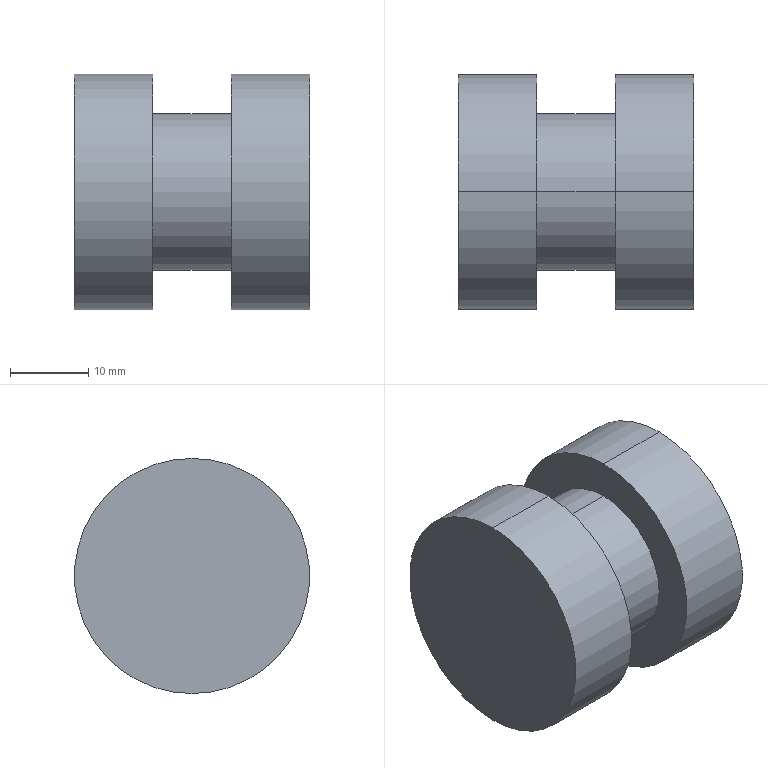Part | SolidWorks | features BaseBody 1 | 1 solid | 10 faces | box 30 x 30 x 30 mm | volume 17279 mm3 | cylinder 6 | plane 4 | commonest cylinder face diameters 30 x4 20 x2
STEP:
#1=CARTESIAN_POINT('',(82.247,407.,68.));
#2=VERTEX_POINT('',#1);
#3=CARTESIAN_POINT('',(82.247,407.,38.));
#4=VERTEX_POINT('',#3);
#5=CARTESIAN_POINT('',(82.247,407.,53.));
#6=DIRECTION('',(-1.,0.,0.));
#7=DIRECTION('',(0.,0.,-1.));
#8=AXIS2_PLACEMENT_3D('',#5,#6,#7);
#9=CIRCLE('',#8,15.);
#10=EDGE_CURVE('',#2,#4,#9,.T.);
#11=ORIENTED_EDGE('',*,*,#10,.F.);
#12=CARTESIAN_POINT('',(92.247,407.,68.));
#13=VERTEX_POINT('',#12);
#14=CARTESIAN_POINT('',(82.247,407.,68.));
#15=DIRECTION('',(1.,0.,0.));
#16=VECTOR('',#15,1000.);
#17=LINE('',#14,#16);
#18=EDGE_CURVE('',#2,#13,#17,.T.);
#19=ORIENTED_EDGE('',*,*,#18,.T.);
#20=CARTESIAN_POINT('',(92.247,407.,38.));
#21=VERTEX_POINT('',#20);
#22=CARTESIAN_POINT('',(92.247,407.,53.));
#23=DIRECTION('',(-1.,0.,0.));
#24=DIRECTION('',(0.,0.,-1.));
#25=AXIS2_PLACEMENT_3D('',#22,#23,#24);
#26=CIRCLE('',#25,15.);
#27=EDGE_CURVE('',#13,#21,#26,.T.);
#28=ORIENTED_EDGE('',*,*,#27,.T.);
#29=CARTESIAN_POINT('',(82.247,407.,38.));
#30=DIRECTION('',(1.,0.,0.));
#31=VECTOR('',#30,1000.);
#32=LINE('',#29,#31);
#33=EDGE_CURVE('',#4,#21,#32,.T.);
#34=ORIENTED_EDGE('',*,*,#33,.F.);
#35=EDGE_LOOP('',(#11,#19,#28,#34));
#36=FACE_OUTER_BOUND('',#35,.T.);
#37=CARTESIAN_POINT('',(82.247,407.,53.));
#38=DIRECTION('',(1.,0.,0.));
#39=DIRECTION('',(0.,0.,-1.));
#40=AXIS2_PLACEMENT_3D('',#37,#38,#39);
#41=CYLINDRICAL_SURFACE('',#40,15.);
#42=ADVANCED_FACE('',(#36),#41,.T.);
#43=CARTESIAN_POINT('',(102.247,407.,63.));
#44=VERTEX_POINT('',#43);
#45=CARTESIAN_POINT('',(102.247,407.,43.));
#46=VERTEX_POINT('',#45);
#47=CARTESIAN_POINT('',(102.247,407.,53.));
#48=DIRECTION('',(-1.,0.,0.));
#49=DIRECTION('',(0.,0.,1.));
#50=AXIS2_PLACEMENT_3D('',#47,#48,#49);
#51=CIRCLE('',#50,10.);
#52=EDGE_CURVE('',#44,#46,#51,.T.);
#53=ORIENTED_EDGE('',*,*,#52,.T.);
#54=CARTESIAN_POINT('',(92.247,407.,43.));
#55=VERTEX_POINT('',#54);
#56=CARTESIAN_POINT('',(102.247,407.,43.));
#57=DIRECTION('',(-1.,0.,0.));
#58=VECTOR('',#57,1000.);
#59=LINE('',#56,#58);
#60=EDGE_CURVE('',#46,#55,#59,.T.);
#61=ORIENTED_EDGE('',*,*,#60,.T.);
#62=CARTESIAN_POINT('',(92.247,407.,63.));
#63=VERTEX_POINT('',#62);
#64=CARTESIAN_POINT('',(92.247,407.,53.));
#65=DIRECTION('',(-1.,0.,0.));
#66=DIRECTION('',(0.,0.,1.));
#67=AXIS2_PLACEMENT_3D('',#64,#65,#66);
#68=CIRCLE('',#67,10.);
#69=EDGE_CURVE('',#63,#55,#68,.T.);
#70=ORIENTED_EDGE('',*,*,#69,.F.);
#71=CARTESIAN_POINT('',(102.247,407.,63.));
#72=DIRECTION('',(-1.,0.,0.));
#73=VECTOR('',#72,1000.);
#74=LINE('',#71,#73);
#75=EDGE_CURVE('',#44,#63,#74,.T.);
#76=ORIENTED_EDGE('',*,*,#75,.F.);
#77=EDGE_LOOP('',(#53,#61,#70,#76));
#78=FACE_OUTER_BOUND('',#77,.T.);
#79=CARTESIAN_POINT('',(102.247,407.,53.));
#80=DIRECTION('',(-1.,0.,0.));
#81=DIRECTION('',(0.,0.,1.));
#82=AXIS2_PLACEMENT_3D('',#79,#80,#81);
#83=CYLINDRICAL_SURFACE('',#82,10.);
#84=ADVANCED_FACE('',(#78),#83,.T.);
#85=CARTESIAN_POINT('',(112.247,407.,68.));
#86=VERTEX_POINT('',#85);
#87=CARTESIAN_POINT('',(112.247,407.,38.));
#88=VERTEX_POINT('',#87);
#89=CARTESIAN_POINT('',(112.247,407.,53.));
#90=DIRECTION('',(-1.,0.,0.));
#91=DIRECTION('',(0.,0.,1.));
#92=AXIS2_PLACEMENT_3D('',#89,#90,#91);
#93=CIRCLE('',#92,15.);
#94=EDGE_CURVE('',#86,#88,#93,.T.);
#95=ORIENTED_EDGE('',*,*,#94,.T.);
#96=CARTESIAN_POINT('',(102.247,407.,38.));
#97=VERTEX_POINT('',#96);
#98=CARTESIAN_POINT('',(112.247,407.,38.));
#99=DIRECTION('',(-1.,0.,0.));
#100=VECTOR('',#99,1000.);
#101=LINE('',#98,#100);
#102=EDGE_CURVE('',#88,#97,#101,.T.);
#103=ORIENTED_EDGE('',*,*,#102,.T.);
#104=CARTESIAN_POINT('',(102.247,407.,68.));
#105=VERTEX_POINT('',#104);
#106=CARTESIAN_POINT('',(102.247,407.,53.));
#107=DIRECTION('',(-1.,0.,0.));
#108=DIRECTION('',(0.,0.,1.));
#109=AXIS2_PLACEMENT_3D('',#106,#107,#108);
#110=CIRCLE('',#109,15.);
#111=EDGE_CURVE('',#105,#97,#110,.T.);
#112=ORIENTED_EDGE('',*,*,#111,.F.);
#113=CARTESIAN_POINT('',(112.247,407.,68.));
#114=DIRECTION('',(-1.,0.,0.));
#115=VECTOR('',#114,1000.);
#116=LINE('',#113,#115);
#117=EDGE_CURVE('',#86,#105,#116,.T.);
#118=ORIENTED_EDGE('',*,*,#117,.F.);
#119=EDGE_LOOP('',(#95,#103,#112,#118));
#120=FACE_OUTER_BOUND('',#119,.T.);
#121=CARTESIAN_POINT('',(112.247,407.,53.));
#122=DIRECTION('',(-1.,0.,0.));
#123=DIRECTION('',(0.,0.,1.));
#124=AXIS2_PLACEMENT_3D('',#121,#122,#123);
#125=CYLINDRICAL_SURFACE('',#124,15.);
#126=ADVANCED_FACE('',(#120),#125,.T.);
#127=CARTESIAN_POINT('',(82.247,407.,53.));
#128=DIRECTION('',(-1.,0.,0.));
#129=DIRECTION('',(0.,0.,-1.));
#130=AXIS2_PLACEMENT_3D('',#127,#128,#129);
#131=CIRCLE('',#130,15.);
#132=EDGE_CURVE('',#4,#2,#131,.T.);
#133=ORIENTED_EDGE('',*,*,#132,.T.);
#134=ORIENTED_EDGE('',*,*,#10,.T.);
#135=EDGE_LOOP('',(#133,#134));
#136=FACE_OUTER_BOUND('',#135,.T.);
#137=CARTESIAN_POINT('',(82.247,407.,53.));
#138=DIRECTION('',(-1.,0.,0.));
#139=DIRECTION('',(0.,0.,1.));
#140=AXIS2_PLACEMENT_3D('',#137,#138,#139);
#141=PLANE('',#140);
#142=ADVANCED_FACE('',(#136),#141,.T.);
#143=ORIENTED_EDGE('',*,*,#18,.F.);
#144=ORIENTED_EDGE('',*,*,#132,.F.);
#145=ORIENTED_EDGE('',*,*,#33,.T.);
#146=CARTESIAN_POINT('',(92.247,407.,53.));
#147=DIRECTION('',(-1.,0.,0.));
#148=DIRECTION('',(0.,0.,-1.));
#149=AXIS2_PLACEMENT_3D('',#146,#147,#148);
#150=CIRCLE('',#149,15.);
#151=EDGE_CURVE('',#21,#13,#150,.T.);
#152=ORIENTED_EDGE('',*,*,#151,.T.);
#153=EDGE_LOOP('',(#143,#144,#145,#152));
#154=FACE_OUTER_BOUND('',#153,.T.);
#155=CARTESIAN_POINT('',(82.247,407.,53.));
#156=DIRECTION('',(1.,0.,0.));
#157=DIRECTION('',(0.,0.,-1.));
#158=AXIS2_PLACEMENT_3D('',#155,#156,#157);
#159=CYLINDRICAL_SURFACE('',#158,15.);
#160=ADVANCED_FACE('',(#154),#159,.T.);
#161=ORIENTED_EDGE('',*,*,#69,.T.);
#162=CARTESIAN_POINT('',(92.247,407.,53.));
#163=DIRECTION('',(-1.,0.,0.));
#164=DIRECTION('',(0.,0.,1.));
#165=AXIS2_PLACEMENT_3D('',#162,#163,#164);
#166=CIRCLE('',#165,10.);
#167=EDGE_CURVE('',#55,#63,#166,.T.);
#168=ORIENTED_EDGE('',*,*,#167,.T.);
#169=EDGE_LOOP('',(#161,#168));
#170=FACE_BOUND('',#169,.T.);
#171=ORIENTED_EDGE('',*,*,#151,.F.);
#172=ORIENTED_EDGE('',*,*,#27,.F.);
#173=EDGE_LOOP('',(#171,#172));
#174=FACE_OUTER_BOUND('',#173,.T.);
#175=CARTESIAN_POINT('',(92.247,407.,53.));
#176=DIRECTION('',(1.,0.,0.));
#177=DIRECTION('',(0.,0.,-1.));
#178=AXIS2_PLACEMENT_3D('',#175,#176,#177);
#179=PLANE('',#178);
#180=ADVANCED_FACE('',(#170,#174),#179,.T.);
#181=ORIENTED_EDGE('',*,*,#60,.F.);
#182=CARTESIAN_POINT('',(102.247,407.,53.));
#183=DIRECTION('',(-1.,0.,0.));
#184=DIRECTION('',(0.,0.,1.));
#185=AXIS2_PLACEMENT_3D('',#182,#183,#184);
#186=CIRCLE('',#185,10.);
#187=EDGE_CURVE('',#46,#44,#186,.T.);
#188=ORIENTED_EDGE('',*,*,#187,.T.);
#189=ORIENTED_EDGE('',*,*,#75,.T.);
#190=ORIENTED_EDGE('',*,*,#167,.F.);
#191=EDGE_LOOP('',(#181,#188,#189,#190));
#192=FACE_OUTER_BOUND('',#191,.T.);
#193=CARTESIAN_POINT('',(102.247,407.,53.));
#194=DIRECTION('',(-1.,0.,0.));
#195=DIRECTION('',(0.,0.,1.));
#196=AXIS2_PLACEMENT_3D('',#193,#194,#195);
#197=CYLINDRICAL_SURFACE('',#196,10.);
#198=ADVANCED_FACE('',(#192),#197,.T.);
#199=ORIENTED_EDGE('',*,*,#52,.F.);
#200=ORIENTED_EDGE('',*,*,#187,.F.);
#201=EDGE_LOOP('',(#199,#200));
#202=FACE_BOUND('',#201,.T.);
#203=ORIENTED_EDGE('',*,*,#111,.T.);
#204=CARTESIAN_POINT('',(102.247,407.,53.));
#205=DIRECTION('',(-1.,0.,0.));
#206=DIRECTION('',(0.,0.,1.));
#207=AXIS2_PLACEMENT_3D('',#204,#205,#206);
#208=CIRCLE('',#207,15.);
#209=EDGE_CURVE('',#97,#105,#208,.T.);
#210=ORIENTED_EDGE('',*,*,#209,.T.);
#211=EDGE_LOOP('',(#203,#210));
#212=FACE_OUTER_BOUND('',#211,.T.);
#213=CARTESIAN_POINT('',(102.247,407.,53.));
#214=DIRECTION('',(-1.,0.,0.));
#215=DIRECTION('',(0.,0.,1.));
#216=AXIS2_PLACEMENT_3D('',#213,#214,#215);
#217=PLANE('',#216);
#218=ADVANCED_FACE('',(#202,#212),#217,.T.);
#219=ORIENTED_EDGE('',*,*,#102,.F.);
#220=CARTESIAN_POINT('',(112.247,407.,53.));
#221=DIRECTION('',(-1.,0.,0.));
#222=DIRECTION('',(0.,0.,1.));
#223=AXIS2_PLACEMENT_3D('',#220,#221,#222);
#224=CIRCLE('',#223,15.);
#225=EDGE_CURVE('',#88,#86,#224,.T.);
#226=ORIENTED_EDGE('',*,*,#225,.T.);
#227=ORIENTED_EDGE('',*,*,#117,.T.);
#228=ORIENTED_EDGE('',*,*,#209,.F.);
#229=EDGE_LOOP('',(#219,#226,#227,#228));
#230=FACE_OUTER_BOUND('',#229,.T.);
#231=CARTESIAN_POINT('',(112.247,407.,53.));
#232=DIRECTION('',(-1.,0.,0.));
#233=DIRECTION('',(0.,0.,1.));
#234=AXIS2_PLACEMENT_3D('',#231,#232,#233);
#235=CYLINDRICAL_SURFACE('',#234,15.);
#236=ADVANCED_FACE('',(#230),#235,.T.);
#237=ORIENTED_EDGE('',*,*,#94,.F.);
#238=ORIENTED_EDGE('',*,*,#225,.F.);
#239=EDGE_LOOP('',(#237,#238));
#240=FACE_OUTER_BOUND('',#239,.T.);
#241=CARTESIAN_POINT('',(112.247,407.,53.));
#242=DIRECTION('',(1.,0.,0.));
#243=DIRECTION('',(0.,0.,-1.));
#244=AXIS2_PLACEMENT_3D('',#241,#242,#243);
#245=PLANE('',#244);
#246=ADVANCED_FACE('',(#240),#245,.T.);
#247=CLOSED_SHELL('',(#42,#84,#126,#142,#160,#180,#198,#218,#236,#246));
#248=MANIFOLD_SOLID_BREP('',#247);
#249=CARTESIAN_POINT('',(0.,0.,0.));
#250=DIRECTION('',(0.,0.,1.));
#251=DIRECTION('',(1.,0.,0.));
#252=AXIS2_PLACEMENT_3D('',#249,#250,#251);
#253=(LENGTH_UNIT()NAMED_UNIT(*)SI_UNIT(.MILLI.,.METRE.));
#254=UNCERTAINTY_MEASURE_WITH_UNIT(LENGTH_MEASURE(0.00001),#253,'','');
#255=(NAMED_UNIT(*)PLANE_ANGLE_UNIT()SI_UNIT($,.RADIAN.));
#256=(NAMED_UNIT(*)SI_UNIT($,.STERADIAN.)SOLID_ANGLE_UNIT());
#257=(GEOMETRIC_REPRESENTATION_CONTEXT(3)GLOBAL_UNCERTAINTY_ASSIGNED_CONTEXT((#254))GLOBAL_UNIT_ASSIGNED_CONTEXT((#253,#255,#256))REPRESENTATION_CONTEXT('',''));
#258=ADVANCED_BREP_SHAPE_REPRESENTATION('',(#248,#252),#257);